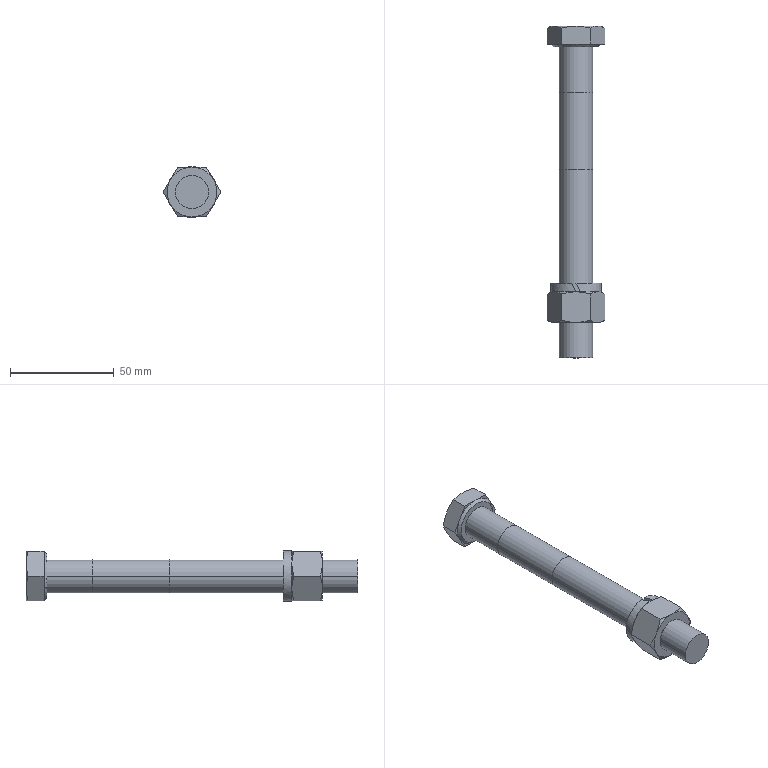Part | NX | features BREP 5, DELETE FACE 1, OFFSET_REGION 1 | 3 solids | 65 faces | box 27.713 x 160 x 24.4 mm | volume 46237 mm3 | plane 29 | cone 24 | cylinder 12 | commonest cylinder face diameters 13.835 x4 16 x4 16.2 x2 24.4 x2